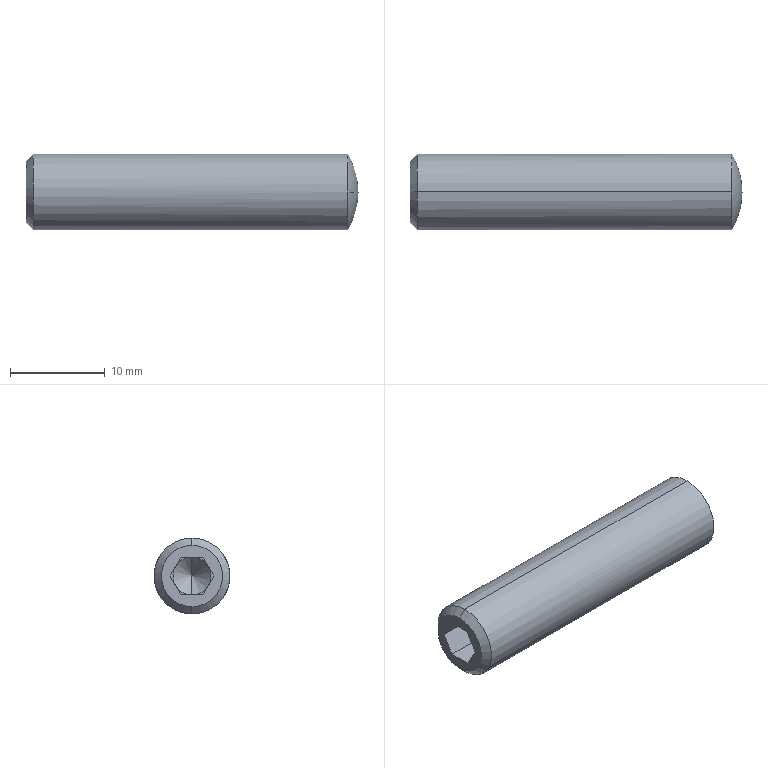Part | STEP file | 1_11 | 1 solid | 21 faces | box 35 x 8 x 8 mm | volume 1662 mm3 | plane 13 | cone 4 | spline 2 | cylinder 2 | commonest cylinder face diameters 8 x2